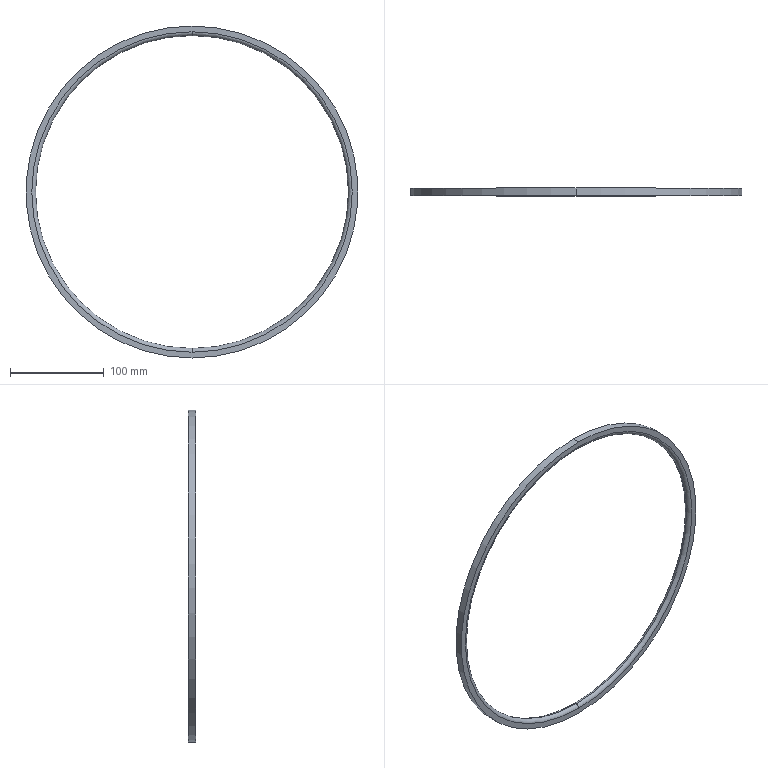Part | SolidWorks | features Revolution 1 | 1 solid | 8 faces | box 354.4 x 8 x 354.4 mm | volume 80993 mm3 | torus 4 | cylinder 2 | plane 2 | commonest cylinder face diameters 354.4 x2
STEP:
#1=CARTESIAN_POINT('',(0.,4.,167.));
#2=VERTEX_POINT('',#1);
#3=CARTESIAN_POINT('',(0.,8.,171.));
#4=VERTEX_POINT('',#3);
#5=CARTESIAN_POINT('',(0.,4.,171.));
#6=DIRECTION('',(1.,0.,0.));
#7=DIRECTION('',(0.,0.,-1.));
#8=AXIS2_PLACEMENT_3D('',#5,#6,#7);
#9=CIRCLE('',#8,4.);
#10=EDGE_CURVE('',#2,#4,#9,.T.);
#11=ORIENTED_EDGE('',*,*,#10,.F.);
#12=CARTESIAN_POINT('',(0.,4.,-167.));
#13=VERTEX_POINT('',#12);
#14=CARTESIAN_POINT('',(0.,4.,0.));
#15=DIRECTION('',(0.,-1.,0.));
#16=DIRECTION('',(0.,0.,-1.));
#17=AXIS2_PLACEMENT_3D('',#14,#15,#16);
#18=CIRCLE('',#17,167.);
#19=EDGE_CURVE('',#2,#13,#18,.T.);
#20=ORIENTED_EDGE('',*,*,#19,.T.);
#21=CARTESIAN_POINT('',(0.,8.,-171.));
#22=VERTEX_POINT('',#21);
#23=CARTESIAN_POINT('',(0.,4.,-171.));
#24=DIRECTION('',(-1.,0.,0.));
#25=DIRECTION('',(0.,0.,1.));
#26=AXIS2_PLACEMENT_3D('',#23,#24,#25);
#27=CIRCLE('',#26,4.);
#28=EDGE_CURVE('',#13,#22,#27,.T.);
#29=ORIENTED_EDGE('',*,*,#28,.T.);
#30=CARTESIAN_POINT('',(0.,8.,0.));
#31=DIRECTION('',(0.,-1.,0.));
#32=DIRECTION('',(0.,0.,-1.));
#33=AXIS2_PLACEMENT_3D('',#30,#31,#32);
#34=CIRCLE('',#33,171.);
#35=EDGE_CURVE('',#4,#22,#34,.T.);
#36=ORIENTED_EDGE('',*,*,#35,.F.);
#37=EDGE_LOOP('',(#11,#20,#29,#36));
#38=FACE_OUTER_BOUND('',#37,.T.);
#39=CARTESIAN_POINT('',(0.,4.,0.));
#40=DIRECTION('',(0.,-1.,0.));
#41=DIRECTION('',(0.,0.,-1.));
#42=AXIS2_PLACEMENT_3D('',#39,#40,#41);
#43=TOROIDAL_SURFACE('',#42,171.,4.);
#44=ADVANCED_FACE('',(#38),#43,.T.);
#45=ORIENTED_EDGE('',*,*,#28,.F.);
#46=CARTESIAN_POINT('',(0.,4.,0.));
#47=DIRECTION('',(0.,-1.,0.));
#48=DIRECTION('',(0.,0.,-1.));
#49=AXIS2_PLACEMENT_3D('',#46,#47,#48);
#50=CIRCLE('',#49,167.);
#51=EDGE_CURVE('',#13,#2,#50,.T.);
#52=ORIENTED_EDGE('',*,*,#51,.T.);
#53=ORIENTED_EDGE('',*,*,#10,.T.);
#54=CARTESIAN_POINT('',(0.,8.,0.));
#55=DIRECTION('',(0.,-1.,0.));
#56=DIRECTION('',(0.,0.,-1.));
#57=AXIS2_PLACEMENT_3D('',#54,#55,#56);
#58=CIRCLE('',#57,171.);
#59=EDGE_CURVE('',#22,#4,#58,.T.);
#60=ORIENTED_EDGE('',*,*,#59,.F.);
#61=EDGE_LOOP('',(#45,#52,#53,#60));
#62=FACE_OUTER_BOUND('',#61,.T.);
#63=CARTESIAN_POINT('',(0.,4.,0.));
#64=DIRECTION('',(0.,-1.,0.));
#65=DIRECTION('',(0.,0.,-1.));
#66=AXIS2_PLACEMENT_3D('',#63,#64,#65);
#67=TOROIDAL_SURFACE('',#66,171.,4.);
#68=ADVANCED_FACE('',(#62),#67,.T.);
#69=CARTESIAN_POINT('',(0.,8.,-177.2));
#70=VERTEX_POINT('',#69);
#71=CARTESIAN_POINT('',(0.,8.,177.2));
#72=VERTEX_POINT('',#71);
#73=CARTESIAN_POINT('',(0.,8.,0.));
#74=DIRECTION('',(0.,-1.,0.));
#75=DIRECTION('',(0.,0.,-1.));
#76=AXIS2_PLACEMENT_3D('',#73,#74,#75);
#77=CIRCLE('',#76,177.2);
#78=EDGE_CURVE('',#70,#72,#77,.T.);
#79=ORIENTED_EDGE('',*,*,#78,.T.);
#80=CARTESIAN_POINT('',(0.,0.,177.2));
#81=VERTEX_POINT('',#80);
#82=CARTESIAN_POINT('',(0.,0.,177.2));
#83=DIRECTION('',(0.,-1.,0.));
#84=VECTOR('',#83,1000.);
#85=LINE('',#82,#84);
#86=EDGE_CURVE('',#72,#81,#85,.T.);
#87=ORIENTED_EDGE('',*,*,#86,.T.);
#88=CARTESIAN_POINT('',(0.,0.,-177.2));
#89=VERTEX_POINT('',#88);
#90=CARTESIAN_POINT('',(0.,0.,0.));
#91=DIRECTION('',(0.,-1.,0.));
#92=DIRECTION('',(0.,0.,-1.));
#93=AXIS2_PLACEMENT_3D('',#90,#91,#92);
#94=CIRCLE('',#93,177.2);
#95=EDGE_CURVE('',#89,#81,#94,.T.);
#96=ORIENTED_EDGE('',*,*,#95,.F.);
#97=CARTESIAN_POINT('',(0.,0.,-177.2));
#98=DIRECTION('',(0.,-1.,0.));
#99=VECTOR('',#98,1000.);
#100=LINE('',#97,#99);
#101=EDGE_CURVE('',#70,#89,#100,.T.);
#102=ORIENTED_EDGE('',*,*,#101,.F.);
#103=EDGE_LOOP('',(#79,#87,#96,#102));
#104=FACE_OUTER_BOUND('',#103,.T.);
#105=CARTESIAN_POINT('',(0.,0.,0.));
#106=DIRECTION('',(0.,-1.,0.));
#107=DIRECTION('',(0.,0.,-1.));
#108=AXIS2_PLACEMENT_3D('',#105,#106,#107);
#109=CYLINDRICAL_SURFACE('',#108,177.2);
#110=ADVANCED_FACE('',(#104),#109,.T.);
#111=ORIENTED_EDGE('',*,*,#51,.F.);
#112=CARTESIAN_POINT('',(0.,0.,-171.));
#113=VERTEX_POINT('',#112);
#114=CARTESIAN_POINT('',(0.,4.,-171.));
#115=DIRECTION('',(-1.,0.,0.));
#116=DIRECTION('',(0.,0.,1.));
#117=AXIS2_PLACEMENT_3D('',#114,#115,#116);
#118=CIRCLE('',#117,4.);
#119=EDGE_CURVE('',#113,#13,#118,.T.);
#120=ORIENTED_EDGE('',*,*,#119,.F.);
#121=CARTESIAN_POINT('',(0.,0.,171.));
#122=VERTEX_POINT('',#121);
#123=CARTESIAN_POINT('',(0.,0.,0.));
#124=DIRECTION('',(0.,-1.,0.));
#125=DIRECTION('',(0.,0.,-1.));
#126=AXIS2_PLACEMENT_3D('',#123,#124,#125);
#127=CIRCLE('',#126,171.);
#128=EDGE_CURVE('',#113,#122,#127,.T.);
#129=ORIENTED_EDGE('',*,*,#128,.T.);
#130=CARTESIAN_POINT('',(0.,4.,171.));
#131=DIRECTION('',(1.,0.,0.));
#132=DIRECTION('',(0.,0.,-1.));
#133=AXIS2_PLACEMENT_3D('',#130,#131,#132);
#134=CIRCLE('',#133,4.);
#135=EDGE_CURVE('',#122,#2,#134,.T.);
#136=ORIENTED_EDGE('',*,*,#135,.T.);
#137=EDGE_LOOP('',(#111,#120,#129,#136));
#138=FACE_OUTER_BOUND('',#137,.T.);
#139=CARTESIAN_POINT('',(0.,4.,0.));
#140=DIRECTION('',(0.,-1.,0.));
#141=DIRECTION('',(0.,0.,-1.));
#142=AXIS2_PLACEMENT_3D('',#139,#140,#141);
#143=TOROIDAL_SURFACE('',#142,171.,4.);
#144=ADVANCED_FACE('',(#138),#143,.T.);
#145=ORIENTED_EDGE('',*,*,#19,.F.);
#146=ORIENTED_EDGE('',*,*,#135,.F.);
#147=CARTESIAN_POINT('',(0.,0.,0.));
#148=DIRECTION('',(0.,-1.,0.));
#149=DIRECTION('',(0.,0.,-1.));
#150=AXIS2_PLACEMENT_3D('',#147,#148,#149);
#151=CIRCLE('',#150,171.);
#152=EDGE_CURVE('',#122,#113,#151,.T.);
#153=ORIENTED_EDGE('',*,*,#152,.T.);
#154=ORIENTED_EDGE('',*,*,#119,.T.);
#155=EDGE_LOOP('',(#145,#146,#153,#154));
#156=FACE_OUTER_BOUND('',#155,.T.);
#157=CARTESIAN_POINT('',(0.,4.,0.));
#158=DIRECTION('',(0.,-1.,0.));
#159=DIRECTION('',(0.,0.,-1.));
#160=AXIS2_PLACEMENT_3D('',#157,#158,#159);
#161=TOROIDAL_SURFACE('',#160,171.,4.);
#162=ADVANCED_FACE('',(#156),#161,.T.);
#163=ORIENTED_EDGE('',*,*,#78,.F.);
#164=CARTESIAN_POINT('',(0.,8.,0.));
#165=DIRECTION('',(0.,-1.,0.));
#166=DIRECTION('',(0.,0.,-1.));
#167=AXIS2_PLACEMENT_3D('',#164,#165,#166);
#168=CIRCLE('',#167,177.2);
#169=EDGE_CURVE('',#72,#70,#168,.T.);
#170=ORIENTED_EDGE('',*,*,#169,.F.);
#171=EDGE_LOOP('',(#163,#170));
#172=FACE_OUTER_BOUND('',#171,.T.);
#173=ORIENTED_EDGE('',*,*,#59,.T.);
#174=ORIENTED_EDGE('',*,*,#35,.T.);
#175=EDGE_LOOP('',(#173,#174));
#176=FACE_BOUND('',#175,.T.);
#177=CARTESIAN_POINT('',(-177.2,8.,0.));
#178=DIRECTION('',(0.,-1.,0.));
#179=DIRECTION('',(0.,0.,-1.));
#180=AXIS2_PLACEMENT_3D('',#177,#178,#179);
#181=PLANE('',#180);
#182=ADVANCED_FACE('',(#172,#176),#181,.F.);
#183=ORIENTED_EDGE('',*,*,#86,.F.);
#184=ORIENTED_EDGE('',*,*,#169,.T.);
#185=ORIENTED_EDGE('',*,*,#101,.T.);
#186=CARTESIAN_POINT('',(0.,0.,0.));
#187=DIRECTION('',(0.,-1.,0.));
#188=DIRECTION('',(0.,0.,-1.));
#189=AXIS2_PLACEMENT_3D('',#186,#187,#188);
#190=CIRCLE('',#189,177.2);
#191=EDGE_CURVE('',#81,#89,#190,.T.);
#192=ORIENTED_EDGE('',*,*,#191,.F.);
#193=EDGE_LOOP('',(#183,#184,#185,#192));
#194=FACE_OUTER_BOUND('',#193,.T.);
#195=CARTESIAN_POINT('',(0.,0.,0.));
#196=DIRECTION('',(0.,-1.,0.));
#197=DIRECTION('',(0.,0.,-1.));
#198=AXIS2_PLACEMENT_3D('',#195,#196,#197);
#199=CYLINDRICAL_SURFACE('',#198,177.2);
#200=ADVANCED_FACE('',(#194),#199,.T.);
#201=ORIENTED_EDGE('',*,*,#128,.F.);
#202=ORIENTED_EDGE('',*,*,#152,.F.);
#203=EDGE_LOOP('',(#201,#202));
#204=FACE_BOUND('',#203,.T.);
#205=ORIENTED_EDGE('',*,*,#95,.T.);
#206=ORIENTED_EDGE('',*,*,#191,.T.);
#207=EDGE_LOOP('',(#205,#206));
#208=FACE_OUTER_BOUND('',#207,.T.);
#209=CARTESIAN_POINT('',(-171.,0.,0.));
#210=DIRECTION('',(0.,1.,0.));
#211=DIRECTION('',(0.,0.,1.));
#212=AXIS2_PLACEMENT_3D('',#209,#210,#211);
#213=PLANE('',#212);
#214=ADVANCED_FACE('',(#204,#208),#213,.F.);
#215=CLOSED_SHELL('',(#44,#68,#110,#144,#162,#182,#200,#214));
#216=MANIFOLD_SOLID_BREP('',#215);
#217=CARTESIAN_POINT('',(0.,0.,0.));
#218=DIRECTION('',(0.,0.,1.));
#219=DIRECTION('',(1.,0.,0.));
#220=AXIS2_PLACEMENT_3D('',#217,#218,#219);
#221=(LENGTH_UNIT()NAMED_UNIT(*)SI_UNIT(.MILLI.,.METRE.));
#222=UNCERTAINTY_MEASURE_WITH_UNIT(LENGTH_MEASURE(0.00001),#221,'','');
#223=(NAMED_UNIT(*)PLANE_ANGLE_UNIT()SI_UNIT($,.RADIAN.));
#224=(NAMED_UNIT(*)SI_UNIT($,.STERADIAN.)SOLID_ANGLE_UNIT());
#225=(GEOMETRIC_REPRESENTATION_CONTEXT(3)GLOBAL_UNCERTAINTY_ASSIGNED_CONTEXT((#222))GLOBAL_UNIT_ASSIGNED_CONTEXT((#221,#223,#224))REPRESENTATION_CONTEXT('',''));
#226=ADVANCED_BREP_SHAPE_REPRESENTATION('',(#216,#220),#225);